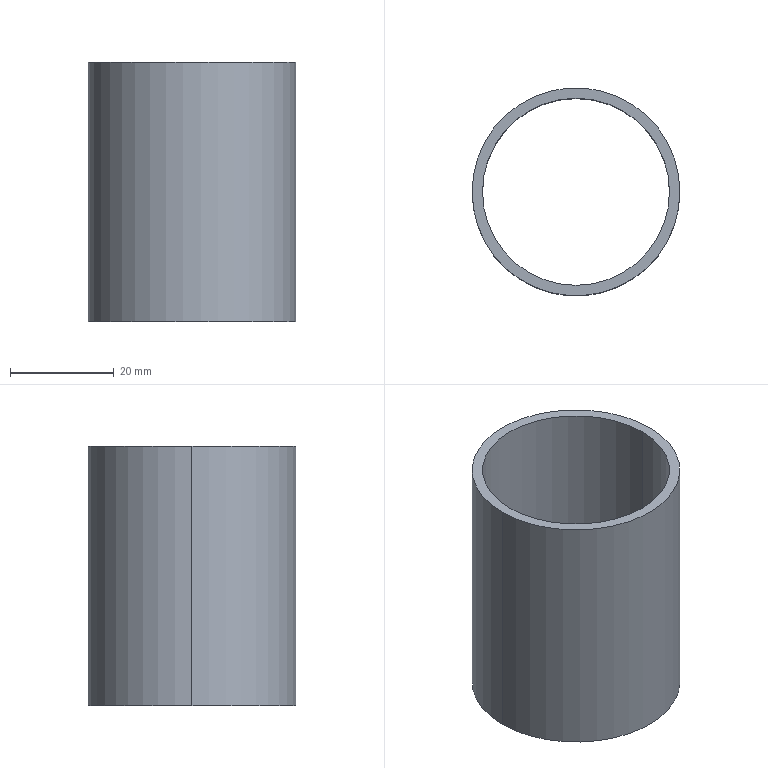Part | SolidWorks | features ICE 3, DeleteBody 2, Split 2, Blend 1, Shell 1 | 1 solid | 6 faces | box 40 x 40 x 50 mm | volume 11938 mm3 | cylinder 4 | plane 2 | commonest cylinder face diameters 36 x2 40 x2
STEP:
#1=CARTESIAN_POINT('',(18.,0.,-400.));
#2=VERTEX_POINT('',#1);
#3=CARTESIAN_POINT('',(-18.,0.,-400.));
#4=VERTEX_POINT('',#3);
#5=CARTESIAN_POINT('',(0.,0.,-400.));
#6=DIRECTION('',(0.,0.,-1.));
#7=DIRECTION('',(-1.,0.,0.));
#8=AXIS2_PLACEMENT_3D('',#5,#6,#7);
#9=CIRCLE('',#8,18.);
#10=EDGE_CURVE('',#2,#4,#9,.T.);
#11=ORIENTED_EDGE('',*,*,#10,.T.);
#12=CARTESIAN_POINT('',(-18.,0.,-350.));
#13=VERTEX_POINT('',#12);
#14=CARTESIAN_POINT('',(-18.,0.,-400.));
#15=DIRECTION('',(0.,0.,1.));
#16=VECTOR('',#15,1000.);
#17=LINE('',#14,#16);
#18=EDGE_CURVE('',#4,#13,#17,.T.);
#19=ORIENTED_EDGE('',*,*,#18,.T.);
#20=CARTESIAN_POINT('',(18.,0.,-350.));
#21=VERTEX_POINT('',#20);
#22=CARTESIAN_POINT('',(0.,0.,-350.));
#23=DIRECTION('',(0.,0.,-1.));
#24=DIRECTION('',(-1.,0.,0.));
#25=AXIS2_PLACEMENT_3D('',#22,#23,#24);
#26=CIRCLE('',#25,18.);
#27=EDGE_CURVE('',#21,#13,#26,.T.);
#28=ORIENTED_EDGE('',*,*,#27,.F.);
#29=CARTESIAN_POINT('',(18.,0.,-400.));
#30=DIRECTION('',(0.,0.,1.));
#31=VECTOR('',#30,1000.);
#32=LINE('',#29,#31);
#33=EDGE_CURVE('',#2,#21,#32,.T.);
#34=ORIENTED_EDGE('',*,*,#33,.F.);
#35=EDGE_LOOP('',(#11,#19,#28,#34));
#36=FACE_OUTER_BOUND('',#35,.T.);
#37=CARTESIAN_POINT('',(0.,0.,-400.));
#38=DIRECTION('',(0.,0.,1.));
#39=DIRECTION('',(1.,0.,0.));
#40=AXIS2_PLACEMENT_3D('',#37,#38,#39);
#41=CYLINDRICAL_SURFACE('',#40,18.);
#42=ADVANCED_FACE('',(#36),#41,.F.);
#43=CARTESIAN_POINT('',(-20.,0.,-400.));
#44=VERTEX_POINT('',#43);
#45=CARTESIAN_POINT('',(20.,0.,-400.));
#46=VERTEX_POINT('',#45);
#47=CARTESIAN_POINT('',(0.,0.,-400.));
#48=DIRECTION('',(0.,0.,-1.));
#49=DIRECTION('',(-1.,0.,0.));
#50=AXIS2_PLACEMENT_3D('',#47,#48,#49);
#51=CIRCLE('',#50,20.);
#52=EDGE_CURVE('',#44,#46,#51,.T.);
#53=ORIENTED_EDGE('',*,*,#52,.F.);
#54=CARTESIAN_POINT('',(-20.,0.,-350.));
#55=VERTEX_POINT('',#54);
#56=CARTESIAN_POINT('',(-20.,0.,-400.));
#57=DIRECTION('',(0.,0.,1.));
#58=VECTOR('',#57,1000.);
#59=LINE('',#56,#58);
#60=EDGE_CURVE('',#44,#55,#59,.T.);
#61=ORIENTED_EDGE('',*,*,#60,.T.);
#62=CARTESIAN_POINT('',(20.,0.,-350.));
#63=VERTEX_POINT('',#62);
#64=CARTESIAN_POINT('',(0.,0.,-350.));
#65=DIRECTION('',(0.,0.,-1.));
#66=DIRECTION('',(1.,0.,0.));
#67=AXIS2_PLACEMENT_3D('',#64,#65,#66);
#68=CIRCLE('',#67,20.);
#69=EDGE_CURVE('',#55,#63,#68,.T.);
#70=ORIENTED_EDGE('',*,*,#69,.T.);
#71=CARTESIAN_POINT('',(20.,0.,-400.));
#72=DIRECTION('',(0.,0.,1.));
#73=VECTOR('',#72,1000.);
#74=LINE('',#71,#73);
#75=EDGE_CURVE('',#46,#63,#74,.T.);
#76=ORIENTED_EDGE('',*,*,#75,.F.);
#77=EDGE_LOOP('',(#53,#61,#70,#76));
#78=FACE_OUTER_BOUND('',#77,.T.);
#79=CARTESIAN_POINT('',(0.,0.,-400.));
#80=DIRECTION('',(0.,0.,1.));
#81=DIRECTION('',(1.,0.,0.));
#82=AXIS2_PLACEMENT_3D('',#79,#80,#81);
#83=CYLINDRICAL_SURFACE('',#82,20.);
#84=ADVANCED_FACE('',(#78),#83,.T.);
#85=ORIENTED_EDGE('',*,*,#27,.T.);
#86=CARTESIAN_POINT('',(0.,0.,-350.));
#87=DIRECTION('',(0.,0.,-1.));
#88=DIRECTION('',(-1.,0.,0.));
#89=AXIS2_PLACEMENT_3D('',#86,#87,#88);
#90=CIRCLE('',#89,18.);
#91=EDGE_CURVE('',#13,#21,#90,.T.);
#92=ORIENTED_EDGE('',*,*,#91,.T.);
#93=EDGE_LOOP('',(#85,#92));
#94=FACE_BOUND('',#93,.T.);
#95=CARTESIAN_POINT('',(0.,0.,-350.));
#96=DIRECTION('',(0.,0.,-1.));
#97=DIRECTION('',(1.,0.,0.));
#98=AXIS2_PLACEMENT_3D('',#95,#96,#97);
#99=CIRCLE('',#98,20.);
#100=EDGE_CURVE('',#63,#55,#99,.T.);
#101=ORIENTED_EDGE('',*,*,#100,.F.);
#102=ORIENTED_EDGE('',*,*,#69,.F.);
#103=EDGE_LOOP('',(#101,#102));
#104=FACE_OUTER_BOUND('',#103,.T.);
#105=CARTESIAN_POINT('',(50.,-50.,-350.));
#106=DIRECTION('',(0.,0.,-1.));
#107=DIRECTION('',(-1.,0.,0.));
#108=AXIS2_PLACEMENT_3D('',#105,#106,#107);
#109=PLANE('',#108);
#110=ADVANCED_FACE('',(#94,#104),#109,.F.);
#111=ORIENTED_EDGE('',*,*,#18,.F.);
#112=CARTESIAN_POINT('',(0.,0.,-400.));
#113=DIRECTION('',(0.,0.,-1.));
#114=DIRECTION('',(-1.,0.,0.));
#115=AXIS2_PLACEMENT_3D('',#112,#113,#114);
#116=CIRCLE('',#115,18.);
#117=EDGE_CURVE('',#4,#2,#116,.T.);
#118=ORIENTED_EDGE('',*,*,#117,.T.);
#119=ORIENTED_EDGE('',*,*,#33,.T.);
#120=ORIENTED_EDGE('',*,*,#91,.F.);
#121=EDGE_LOOP('',(#111,#118,#119,#120));
#122=FACE_OUTER_BOUND('',#121,.T.);
#123=CARTESIAN_POINT('',(0.,0.,-400.));
#124=DIRECTION('',(0.,0.,1.));
#125=DIRECTION('',(1.,0.,0.));
#126=AXIS2_PLACEMENT_3D('',#123,#124,#125);
#127=CYLINDRICAL_SURFACE('',#126,18.);
#128=ADVANCED_FACE('',(#122),#127,.F.);
#129=ORIENTED_EDGE('',*,*,#60,.F.);
#130=CARTESIAN_POINT('',(0.,0.,-400.));
#131=DIRECTION('',(0.,0.,-1.));
#132=DIRECTION('',(-1.,0.,0.));
#133=AXIS2_PLACEMENT_3D('',#130,#131,#132);
#134=CIRCLE('',#133,20.);
#135=EDGE_CURVE('',#46,#44,#134,.T.);
#136=ORIENTED_EDGE('',*,*,#135,.F.);
#137=ORIENTED_EDGE('',*,*,#75,.T.);
#138=ORIENTED_EDGE('',*,*,#100,.T.);
#139=EDGE_LOOP('',(#129,#136,#137,#138));
#140=FACE_OUTER_BOUND('',#139,.T.);
#141=CARTESIAN_POINT('',(0.,0.,-400.));
#142=DIRECTION('',(0.,0.,1.));
#143=DIRECTION('',(1.,0.,0.));
#144=AXIS2_PLACEMENT_3D('',#141,#142,#143);
#145=CYLINDRICAL_SURFACE('',#144,20.);
#146=ADVANCED_FACE('',(#140),#145,.T.);
#147=ORIENTED_EDGE('',*,*,#135,.T.);
#148=ORIENTED_EDGE('',*,*,#52,.T.);
#149=EDGE_LOOP('',(#147,#148));
#150=FACE_OUTER_BOUND('',#149,.T.);
#151=ORIENTED_EDGE('',*,*,#10,.F.);
#152=ORIENTED_EDGE('',*,*,#117,.F.);
#153=EDGE_LOOP('',(#151,#152));
#154=FACE_BOUND('',#153,.T.);
#155=CARTESIAN_POINT('',(0.,0.,-400.));
#156=DIRECTION('',(0.,0.,-1.));
#157=DIRECTION('',(-1.,0.,0.));
#158=AXIS2_PLACEMENT_3D('',#155,#156,#157);
#159=PLANE('',#158);
#160=ADVANCED_FACE('',(#150,#154),#159,.T.);
#161=CLOSED_SHELL('',(#42,#84,#110,#128,#146,#160));
#162=MANIFOLD_SOLID_BREP('',#161);
#163=CARTESIAN_POINT('',(0.,0.,0.));
#164=DIRECTION('',(0.,0.,1.));
#165=DIRECTION('',(1.,0.,0.));
#166=AXIS2_PLACEMENT_3D('',#163,#164,#165);
#167=(LENGTH_UNIT()NAMED_UNIT(*)SI_UNIT(.MILLI.,.METRE.));
#168=UNCERTAINTY_MEASURE_WITH_UNIT(LENGTH_MEASURE(0.00001),#167,'','');
#169=(NAMED_UNIT(*)PLANE_ANGLE_UNIT()SI_UNIT($,.RADIAN.));
#170=(NAMED_UNIT(*)SI_UNIT($,.STERADIAN.)SOLID_ANGLE_UNIT());
#171=(GEOMETRIC_REPRESENTATION_CONTEXT(3)GLOBAL_UNCERTAINTY_ASSIGNED_CONTEXT((#168))GLOBAL_UNIT_ASSIGNED_CONTEXT((#167,#169,#170))REPRESENTATION_CONTEXT('',''));
#172=ADVANCED_BREP_SHAPE_REPRESENTATION('',(#162,#166),#171);